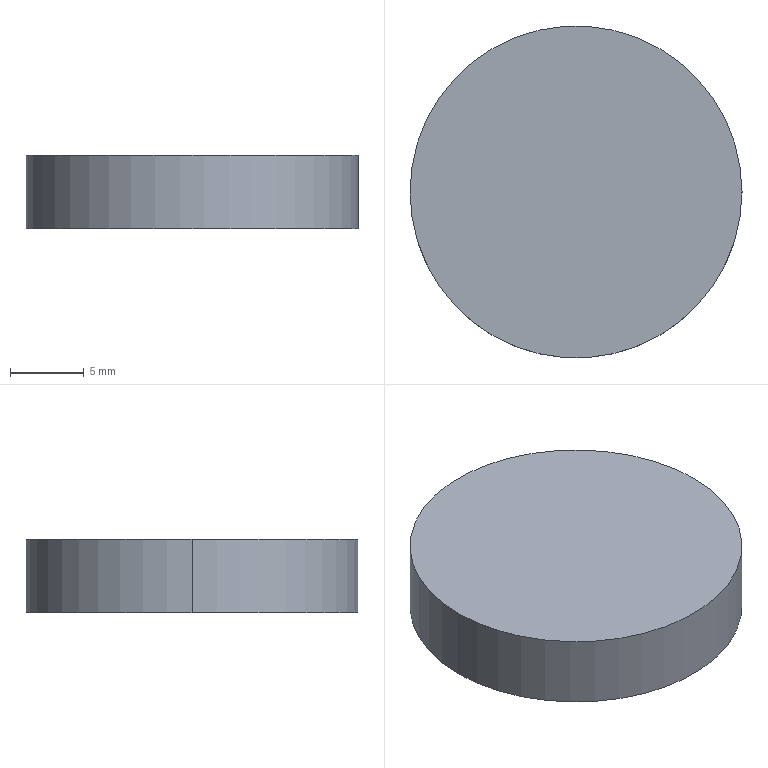Part | STEP file | Buzzer large | 1 solid | 4 faces | box 22.5 x 22.5 x 5 mm | volume 1988 mm3 | cylinder 2 | plane 2 | commonest cylinder face diameters 22.5 x2
STEP:
#1=CARTESIAN_POINT('',(0.,0.,0.));
#2=DIRECTION('',(0.,0.,1.));
#3=DIRECTION('',(1.,0.,0.));
#4=AXIS2_PLACEMENT_3D('',#1,#2,#3);
#5=CARTESIAN_POINT('',(11.25,0.,5.));
#6=VERTEX_POINT('',#5);
#7=CARTESIAN_POINT('',(-11.25,0.,5.));
#8=VERTEX_POINT('',#7);
#9=CARTESIAN_POINT('',(0.,0.,5.));
#10=DIRECTION('',(0.,0.,1.));
#11=DIRECTION('',(-1.,0.,0.));
#12=AXIS2_PLACEMENT_3D('',#9,#10,#11);
#13=CIRCLE('',#12,11.25);
#14=CARTESIAN_POINT('',(0.,0.,5.));
#15=DIRECTION('',(0.,0.,-1.));
#16=DIRECTION('',(-1.,0.,0.));
#17=AXIS2_PLACEMENT_3D('',#14,#15,#16);
#18=CYLINDRICAL_SURFACE('',#17,11.25);
#19=CARTESIAN_POINT('',(6.283,0.));
#20=DIRECTION('',(-1.,0.));
#21=VECTOR('',#20,1.);
#22=LINE('',#19,#21);
#23=(GEOMETRIC_REPRESENTATION_CONTEXT(2)PARAMETRIC_REPRESENTATION_CONTEXT()REPRESENTATION_CONTEXT('',''));
#24=DEFINITIONAL_REPRESENTATION('',(#22),#23);
#25=PCURVE('',#18,#24);
#26=CARTESIAN_POINT('',(0.,0.,5.));
#27=DIRECTION('',(0.,0.,1.));
#28=DIRECTION('',(1.,0.,0.));
#29=AXIS2_PLACEMENT_3D('',#26,#27,#28);
#30=PLANE('',#29);
#31=CARTESIAN_POINT('',(0.,0.));
#32=DIRECTION('',(-1.,0.));
#33=AXIS2_PLACEMENT_2D('',#31,#32);
#34=CIRCLE('',#33,11.25);
#35=(GEOMETRIC_REPRESENTATION_CONTEXT(2)PARAMETRIC_REPRESENTATION_CONTEXT()REPRESENTATION_CONTEXT('',''));
#36=DEFINITIONAL_REPRESENTATION('',(#34),#35);
#37=PCURVE('',#30,#36);
#38=SURFACE_CURVE('',#13,(#25,#37),.PCURVE_S1.);
#39=EDGE_CURVE('',#6,#8,#38,.T.);
#40=ORIENTED_EDGE('',*,*,#39,.F.);
#41=CARTESIAN_POINT('',(11.25,0.,0.));
#42=VERTEX_POINT('',#41);
#43=CARTESIAN_POINT('',(11.25,0.,5.));
#44=DIRECTION('',(0.,0.,-1.));
#45=VECTOR('',#44,1.);
#46=LINE('',#43,#45);
#47=CARTESIAN_POINT('',(3.142,0.));
#48=DIRECTION('',(0.,1.));
#49=VECTOR('',#48,1.);
#50=LINE('',#47,#49);
#51=(GEOMETRIC_REPRESENTATION_CONTEXT(2)PARAMETRIC_REPRESENTATION_CONTEXT()REPRESENTATION_CONTEXT('',''));
#52=DEFINITIONAL_REPRESENTATION('',(#50),#51);
#53=PCURVE('',#18,#52);
#54=CARTESIAN_POINT('',(0.,0.,5.));
#55=DIRECTION('',(0.,0.,-1.));
#56=DIRECTION('',(-1.,0.,0.));
#57=AXIS2_PLACEMENT_3D('',#54,#55,#56);
#58=CYLINDRICAL_SURFACE('',#57,11.25);
#59=CARTESIAN_POINT('',(3.142,0.));
#60=DIRECTION('',(0.,1.));
#61=VECTOR('',#60,1.);
#62=LINE('',#59,#61);
#63=(GEOMETRIC_REPRESENTATION_CONTEXT(2)PARAMETRIC_REPRESENTATION_CONTEXT()REPRESENTATION_CONTEXT('',''));
#64=DEFINITIONAL_REPRESENTATION('',(#62),#63);
#65=PCURVE('',#58,#64);
#66=SURFACE_CURVE('',#46,(#53,#65),.PCURVE_S1.);
#67=EDGE_CURVE('',#6,#42,#66,.T.);
#68=ORIENTED_EDGE('',*,*,#67,.T.);
#69=CARTESIAN_POINT('',(-11.25,0.,0.));
#70=VERTEX_POINT('',#69);
#71=CARTESIAN_POINT('',(0.,0.,0.));
#72=DIRECTION('',(0.,0.,1.));
#73=DIRECTION('',(-1.,0.,0.));
#74=AXIS2_PLACEMENT_3D('',#71,#72,#73);
#75=CIRCLE('',#74,11.25);
#76=CARTESIAN_POINT('',(6.283,5.));
#77=DIRECTION('',(-1.,0.));
#78=VECTOR('',#77,1.);
#79=LINE('',#76,#78);
#80=(GEOMETRIC_REPRESENTATION_CONTEXT(2)PARAMETRIC_REPRESENTATION_CONTEXT()REPRESENTATION_CONTEXT('',''));
#81=DEFINITIONAL_REPRESENTATION('',(#79),#80);
#82=PCURVE('',#18,#81);
#83=CARTESIAN_POINT('',(0.,0.,0.));
#84=DIRECTION('',(0.,0.,1.));
#85=DIRECTION('',(1.,0.,0.));
#86=AXIS2_PLACEMENT_3D('',#83,#84,#85);
#87=PLANE('',#86);
#88=CARTESIAN_POINT('',(0.,0.));
#89=DIRECTION('',(-1.,0.));
#90=AXIS2_PLACEMENT_2D('',#88,#89);
#91=CIRCLE('',#90,11.25);
#92=(GEOMETRIC_REPRESENTATION_CONTEXT(2)PARAMETRIC_REPRESENTATION_CONTEXT()REPRESENTATION_CONTEXT('',''));
#93=DEFINITIONAL_REPRESENTATION('',(#91),#92);
#94=PCURVE('',#87,#93);
#95=SURFACE_CURVE('',#75,(#82,#94),.PCURVE_S1.);
#96=EDGE_CURVE('',#42,#70,#95,.T.);
#97=ORIENTED_EDGE('',*,*,#96,.T.);
#98=CARTESIAN_POINT('',(-11.25,0.,5.));
#99=DIRECTION('',(0.,0.,-1.));
#100=VECTOR('',#99,1.);
#101=LINE('',#98,#100);
#102=CARTESIAN_POINT('',(0.,0.));
#103=DIRECTION('',(0.,1.));
#104=VECTOR('',#103,1.);
#105=LINE('',#102,#104);
#106=(GEOMETRIC_REPRESENTATION_CONTEXT(2)PARAMETRIC_REPRESENTATION_CONTEXT()REPRESENTATION_CONTEXT('',''));
#107=DEFINITIONAL_REPRESENTATION('',(#105),#106);
#108=PCURVE('',#18,#107);
#109=CARTESIAN_POINT('',(6.283,0.));
#110=DIRECTION('',(0.,1.));
#111=VECTOR('',#110,1.);
#112=LINE('',#109,#111);
#113=(GEOMETRIC_REPRESENTATION_CONTEXT(2)PARAMETRIC_REPRESENTATION_CONTEXT()REPRESENTATION_CONTEXT('',''));
#114=DEFINITIONAL_REPRESENTATION('',(#112),#113);
#115=PCURVE('',#58,#114);
#116=SURFACE_CURVE('',#101,(#108,#115),.PCURVE_S1.);
#117=EDGE_CURVE('',#8,#70,#116,.T.);
#118=ORIENTED_EDGE('',*,*,#117,.F.);
#119=EDGE_LOOP('',(#40,#68,#97,#118));
#120=FACE_BOUND('',#119,.T.);
#121=ADVANCED_FACE('',(#120),#18,.T.);
#122=CARTESIAN_POINT('',(0.,0.,5.));
#123=DIRECTION('',(0.,0.,1.));
#124=DIRECTION('',(-1.,0.,0.));
#125=AXIS2_PLACEMENT_3D('',#122,#123,#124);
#126=CIRCLE('',#125,11.25);
#127=CARTESIAN_POINT('',(0.,0.));
#128=DIRECTION('',(-1.,0.));
#129=AXIS2_PLACEMENT_2D('',#127,#128);
#130=CIRCLE('',#129,11.25);
#131=(GEOMETRIC_REPRESENTATION_CONTEXT(2)PARAMETRIC_REPRESENTATION_CONTEXT()REPRESENTATION_CONTEXT('',''));
#132=DEFINITIONAL_REPRESENTATION('',(#130),#131);
#133=PCURVE('',#30,#132);
#134=CARTESIAN_POINT('',(6.283,0.));
#135=DIRECTION('',(-1.,0.));
#136=VECTOR('',#135,1.);
#137=LINE('',#134,#136);
#138=(GEOMETRIC_REPRESENTATION_CONTEXT(2)PARAMETRIC_REPRESENTATION_CONTEXT()REPRESENTATION_CONTEXT('',''));
#139=DEFINITIONAL_REPRESENTATION('',(#137),#138);
#140=PCURVE('',#58,#139);
#141=SURFACE_CURVE('',#126,(#133,#140),.PCURVE_S1.);
#142=EDGE_CURVE('',#8,#6,#141,.T.);
#143=ORIENTED_EDGE('',*,*,#142,.T.);
#144=ORIENTED_EDGE('',*,*,#39,.T.);
#145=EDGE_LOOP('',(#143,#144));
#146=FACE_BOUND('',#145,.T.);
#147=ADVANCED_FACE('',(#146),#30,.T.);
#148=ORIENTED_EDGE('',*,*,#67,.F.);
#149=ORIENTED_EDGE('',*,*,#142,.F.);
#150=ORIENTED_EDGE('',*,*,#117,.T.);
#151=CARTESIAN_POINT('',(0.,0.,0.));
#152=DIRECTION('',(0.,0.,1.));
#153=DIRECTION('',(-1.,0.,0.));
#154=AXIS2_PLACEMENT_3D('',#151,#152,#153);
#155=CIRCLE('',#154,11.25);
#156=CARTESIAN_POINT('',(6.283,5.));
#157=DIRECTION('',(-1.,0.));
#158=VECTOR('',#157,1.);
#159=LINE('',#156,#158);
#160=(GEOMETRIC_REPRESENTATION_CONTEXT(2)PARAMETRIC_REPRESENTATION_CONTEXT()REPRESENTATION_CONTEXT('',''));
#161=DEFINITIONAL_REPRESENTATION('',(#159),#160);
#162=PCURVE('',#58,#161);
#163=CARTESIAN_POINT('',(0.,0.));
#164=DIRECTION('',(-1.,0.));
#165=AXIS2_PLACEMENT_2D('',#163,#164);
#166=CIRCLE('',#165,11.25);
#167=(GEOMETRIC_REPRESENTATION_CONTEXT(2)PARAMETRIC_REPRESENTATION_CONTEXT()REPRESENTATION_CONTEXT('',''));
#168=DEFINITIONAL_REPRESENTATION('',(#166),#167);
#169=PCURVE('',#87,#168);
#170=SURFACE_CURVE('',#155,(#162,#169),.PCURVE_S1.);
#171=EDGE_CURVE('',#70,#42,#170,.T.);
#172=ORIENTED_EDGE('',*,*,#171,.T.);
#173=EDGE_LOOP('',(#148,#149,#150,#172));
#174=FACE_BOUND('',#173,.T.);
#175=ADVANCED_FACE('',(#174),#58,.T.);
#176=ORIENTED_EDGE('',*,*,#171,.F.);
#177=ORIENTED_EDGE('',*,*,#96,.F.);
#178=EDGE_LOOP('',(#176,#177));
#179=FACE_BOUND('',#178,.T.);
#180=ADVANCED_FACE('',(#179),#87,.F.);
#181=CLOSED_SHELL('',(#121,#147,#175,#180));
#182=MANIFOLD_SOLID_BREP('',#181);
#183=(LENGTH_UNIT()NAMED_UNIT(*)SI_UNIT(.MILLI.,.METRE.));
#184=UNCERTAINTY_MEASURE_WITH_UNIT(LENGTH_MEASURE(0.0000001),#183,'','');
#185=(NAMED_UNIT(*)PLANE_ANGLE_UNIT()SI_UNIT($,.RADIAN.));
#186=(NAMED_UNIT(*)SI_UNIT($,.STERADIAN.)SOLID_ANGLE_UNIT());
#187=(GEOMETRIC_REPRESENTATION_CONTEXT(3)GLOBAL_UNCERTAINTY_ASSIGNED_CONTEXT((#184))GLOBAL_UNIT_ASSIGNED_CONTEXT((#183,#185,#186))REPRESENTATION_CONTEXT('',''));
#188=ADVANCED_BREP_SHAPE_REPRESENTATION('',(#4,#182),#187);